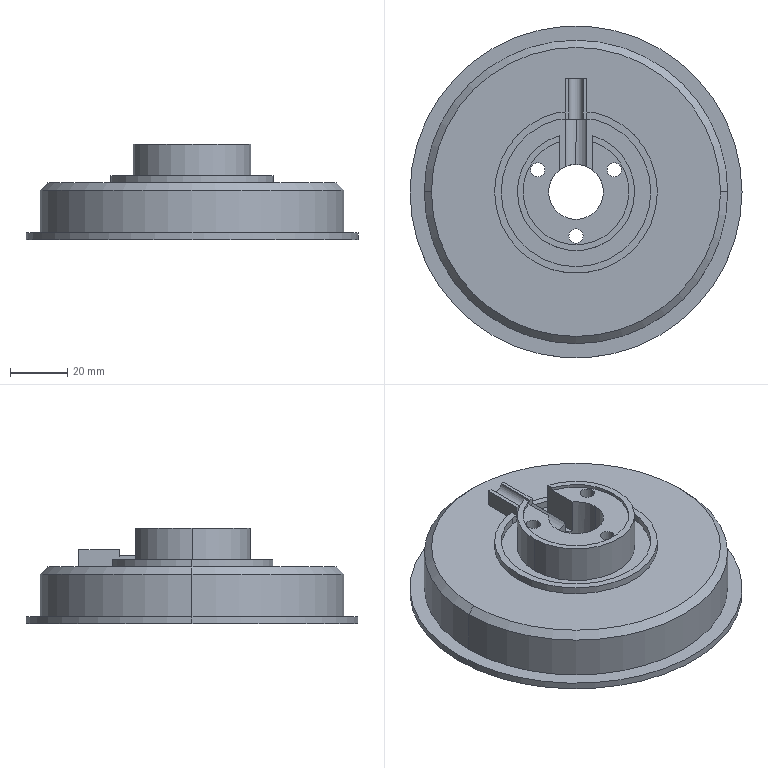Part | SolidWorks | features ICE 11, Chamfer 1, Extrusion 1 | 1 solid | 71 faces | box 116 x 116 x 33.3 mm | volume 52599 mm3 | cylinder 37 | plane 32 | cone 2 | commonest cylinder face diameters 37 x8 5 x7 23.5 x3 41 x3 52.3 x3 56.9 x3